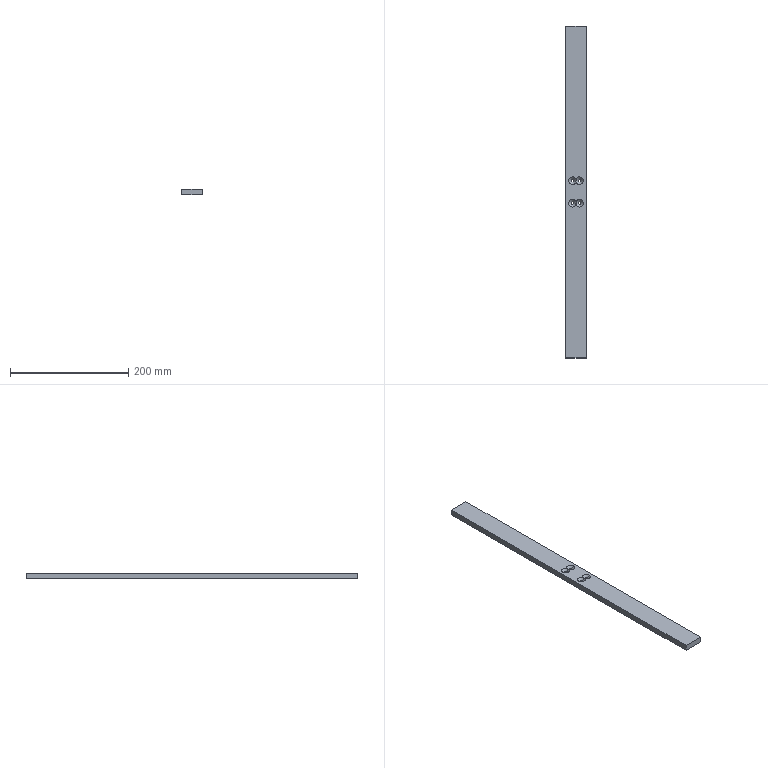Part | STEP file | 1 solid | 22 faces | box 35 x 562 x 10 mm | volume 195044 mm3 | cylinder 8 | cone 8 | plane 6 | commonest cylinder face diameters 5.5 x8